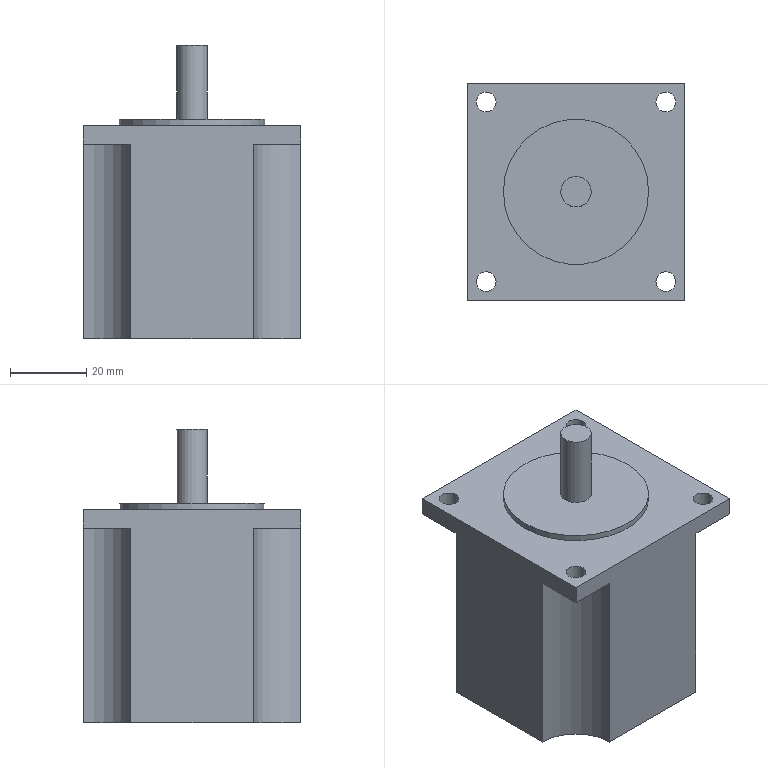Part | NX | features 57BYG350CL-SASSML-0601步进电机.SLDPRT 2 | 1 solid | 22 faces | box 57 x 57 x 76.9 mm | volume 158968 mm3 | plane 12 | cylinder 10 | commonest cylinder face diameters 5.2 x4 25 x4 8 x1 38.1 x1
STEP:
#1=CARTESIAN_POINT('',(-36.836,-5.583,23.));
#2=VERTEX_POINT('',#1);
#3=CARTESIAN_POINT('',(-36.836,26.417,23.));
#4=VERTEX_POINT('',#3);
#5=CARTESIAN_POINT('',(-36.836,38.917,23.));
#6=DIRECTION('',(0.,1.,0.));
#7=VECTOR('',#6,1000.);
#8=LINE('',#5,#7);
#9=EDGE_CURVE('',#2,#4,#8,.T.);
#10=ORIENTED_EDGE('',*,*,#9,.F.);
#11=CARTESIAN_POINT('',(-36.836,-5.583,74.));
#12=VERTEX_POINT('',#11);
#13=CARTESIAN_POINT('',(-36.836,-5.583,74.));
#14=DIRECTION('',(0.,0.,-1.));
#15=VECTOR('',#14,1000.);
#16=LINE('',#13,#15);
#17=EDGE_CURVE('',#2,#12,#16,.F.);
#18=ORIENTED_EDGE('',*,*,#17,.T.);
#19=CARTESIAN_POINT('',(-36.836,-18.083,74.));
#20=VERTEX_POINT('',#19);
#21=CARTESIAN_POINT('',(-36.836,-18.083,74.));
#22=DIRECTION('',(0.,1.,0.));
#23=VECTOR('',#22,1000.);
#24=LINE('',#21,#23);
#25=EDGE_CURVE('',#20,#12,#24,.T.);
#26=ORIENTED_EDGE('',*,*,#25,.F.);
#27=CARTESIAN_POINT('',(-36.836,-18.083,78.9));
#28=VERTEX_POINT('',#27);
#29=CARTESIAN_POINT('',(-36.836,-18.083,78.9));
#30=DIRECTION('',(0.,0.,-1.));
#31=VECTOR('',#30,1000.);
#32=LINE('',#29,#31);
#33=EDGE_CURVE('',#28,#20,#32,.T.);
#34=ORIENTED_EDGE('',*,*,#33,.F.);
#35=CARTESIAN_POINT('',(-36.836,38.917,78.9));
#36=VERTEX_POINT('',#35);
#37=CARTESIAN_POINT('',(-36.836,-18.083,78.9));
#38=DIRECTION('',(0.,-1.,0.));
#39=VECTOR('',#38,1000.);
#40=LINE('',#37,#39);
#41=EDGE_CURVE('',#36,#28,#40,.T.);
#42=ORIENTED_EDGE('',*,*,#41,.F.);
#43=CARTESIAN_POINT('',(-36.836,38.917,74.));
#44=VERTEX_POINT('',#43);
#45=CARTESIAN_POINT('',(-36.836,38.917,78.9));
#46=DIRECTION('',(0.,0.,-1.));
#47=VECTOR('',#46,1000.);
#48=LINE('',#45,#47);
#49=EDGE_CURVE('',#36,#44,#48,.T.);
#50=ORIENTED_EDGE('',*,*,#49,.T.);
#51=CARTESIAN_POINT('',(-36.836,26.417,74.));
#52=VERTEX_POINT('',#51);
#53=CARTESIAN_POINT('',(-36.836,-18.083,74.));
#54=DIRECTION('',(0.,1.,0.));
#55=VECTOR('',#54,1000.);
#56=LINE('',#53,#55);
#57=EDGE_CURVE('',#52,#44,#56,.T.);
#58=ORIENTED_EDGE('',*,*,#57,.F.);
#59=CARTESIAN_POINT('',(-36.836,26.417,74.));
#60=DIRECTION('',(0.,0.,-1.));
#61=VECTOR('',#60,1000.);
#62=LINE('',#59,#61);
#63=EDGE_CURVE('',#52,#4,#62,.T.);
#64=ORIENTED_EDGE('',*,*,#63,.T.);
#65=EDGE_LOOP('',(#10,#18,#26,#34,#42,#50,#58,#64));
#66=FACE_BOUND('',#65,.T.);
#67=CARTESIAN_POINT('',(-36.836,-18.083,78.9));
#68=DIRECTION('',(1.,0.,0.));
#69=DIRECTION('',(0.,0.,-1.));
#70=AXIS2_PLACEMENT_3D('',#67,#68,#69);
#71=PLANE('',#70);
#72=ADVANCED_FACE('',(#66),#71,.F.);
#73=CARTESIAN_POINT('',(7.664,-18.083,23.));
#74=VERTEX_POINT('',#73);
#75=CARTESIAN_POINT('',(-24.336,-18.083,23.));
#76=VERTEX_POINT('',#75);
#77=CARTESIAN_POINT('',(20.164,-18.083,23.));
#78=DIRECTION('',(-1.,0.,0.));
#79=VECTOR('',#78,1000.);
#80=LINE('',#77,#79);
#81=EDGE_CURVE('',#74,#76,#80,.T.);
#82=ORIENTED_EDGE('',*,*,#81,.F.);
#83=CARTESIAN_POINT('',(7.664,-18.083,74.));
#84=VERTEX_POINT('',#83);
#85=CARTESIAN_POINT('',(7.664,-18.083,74.));
#86=DIRECTION('',(0.,0.,-1.));
#87=VECTOR('',#86,1000.);
#88=LINE('',#85,#87);
#89=EDGE_CURVE('',#74,#84,#88,.F.);
#90=ORIENTED_EDGE('',*,*,#89,.T.);
#91=CARTESIAN_POINT('',(20.164,-18.083,74.));
#92=VERTEX_POINT('',#91);
#93=CARTESIAN_POINT('',(-36.836,-18.083,74.));
#94=DIRECTION('',(-1.,0.,0.));
#95=VECTOR('',#94,1000.);
#96=LINE('',#93,#95);
#97=EDGE_CURVE('',#92,#84,#96,.T.);
#98=ORIENTED_EDGE('',*,*,#97,.F.);
#99=CARTESIAN_POINT('',(20.164,-18.083,78.9));
#100=VERTEX_POINT('',#99);
#101=CARTESIAN_POINT('',(20.164,-18.083,78.9));
#102=DIRECTION('',(0.,0.,-1.));
#103=VECTOR('',#102,1000.);
#104=LINE('',#101,#103);
#105=EDGE_CURVE('',#100,#92,#104,.T.);
#106=ORIENTED_EDGE('',*,*,#105,.F.);
#107=CARTESIAN_POINT('',(-36.836,-18.083,78.9));
#108=DIRECTION('',(1.,0.,0.));
#109=VECTOR('',#108,1000.);
#110=LINE('',#107,#109);
#111=EDGE_CURVE('',#28,#100,#110,.T.);
#112=ORIENTED_EDGE('',*,*,#111,.F.);
#113=ORIENTED_EDGE('',*,*,#33,.T.);
#114=CARTESIAN_POINT('',(-24.336,-18.083,74.));
#115=VERTEX_POINT('',#114);
#116=CARTESIAN_POINT('',(-36.836,-18.083,74.));
#117=DIRECTION('',(-1.,0.,0.));
#118=VECTOR('',#117,1000.);
#119=LINE('',#116,#118);
#120=EDGE_CURVE('',#115,#20,#119,.T.);
#121=ORIENTED_EDGE('',*,*,#120,.F.);
#122=CARTESIAN_POINT('',(-24.336,-18.083,74.));
#123=DIRECTION('',(0.,0.,-1.));
#124=VECTOR('',#123,1000.);
#125=LINE('',#122,#124);
#126=EDGE_CURVE('',#115,#76,#125,.T.);
#127=ORIENTED_EDGE('',*,*,#126,.T.);
#128=EDGE_LOOP('',(#82,#90,#98,#106,#112,#113,#121,#127));
#129=FACE_BOUND('',#128,.T.);
#130=CARTESIAN_POINT('',(-36.836,-18.083,78.9));
#131=DIRECTION('',(0.,1.,0.));
#132=DIRECTION('',(0.,0.,1.));
#133=AXIS2_PLACEMENT_3D('',#130,#131,#132);
#134=PLANE('',#133);
#135=ADVANCED_FACE('',(#129),#134,.F.);
#136=CARTESIAN_POINT('',(20.164,26.417,23.));
#137=VERTEX_POINT('',#136);
#138=CARTESIAN_POINT('',(20.164,-5.583,23.));
#139=VERTEX_POINT('',#138);
#140=CARTESIAN_POINT('',(20.164,38.917,23.));
#141=DIRECTION('',(0.,-1.,0.));
#142=VECTOR('',#141,1000.);
#143=LINE('',#140,#142);
#144=EDGE_CURVE('',#137,#139,#143,.T.);
#145=ORIENTED_EDGE('',*,*,#144,.F.);
#146=CARTESIAN_POINT('',(20.164,26.417,74.));
#147=VERTEX_POINT('',#146);
#148=CARTESIAN_POINT('',(20.164,26.417,74.));
#149=DIRECTION('',(0.,0.,-1.));
#150=VECTOR('',#149,1000.);
#151=LINE('',#148,#150);
#152=EDGE_CURVE('',#137,#147,#151,.F.);
#153=ORIENTED_EDGE('',*,*,#152,.T.);
#154=CARTESIAN_POINT('',(20.164,38.917,74.));
#155=VERTEX_POINT('',#154);
#156=CARTESIAN_POINT('',(20.164,-18.083,74.));
#157=DIRECTION('',(0.,-1.,0.));
#158=VECTOR('',#157,1000.);
#159=LINE('',#156,#158);
#160=EDGE_CURVE('',#155,#147,#159,.T.);
#161=ORIENTED_EDGE('',*,*,#160,.F.);
#162=CARTESIAN_POINT('',(20.164,38.917,78.9));
#163=VERTEX_POINT('',#162);
#164=CARTESIAN_POINT('',(20.164,38.917,78.9));
#165=DIRECTION('',(0.,0.,-1.));
#166=VECTOR('',#165,1000.);
#167=LINE('',#164,#166);
#168=EDGE_CURVE('',#163,#155,#167,.T.);
#169=ORIENTED_EDGE('',*,*,#168,.F.);
#170=CARTESIAN_POINT('',(20.164,-18.083,78.9));
#171=DIRECTION('',(0.,1.,0.));
#172=VECTOR('',#171,1000.);
#173=LINE('',#170,#172);
#174=EDGE_CURVE('',#100,#163,#173,.T.);
#175=ORIENTED_EDGE('',*,*,#174,.F.);
#176=ORIENTED_EDGE('',*,*,#105,.T.);
#177=CARTESIAN_POINT('',(20.164,-5.583,74.));
#178=VERTEX_POINT('',#177);
#179=CARTESIAN_POINT('',(20.164,-18.083,74.));
#180=DIRECTION('',(0.,-1.,0.));
#181=VECTOR('',#180,1000.);
#182=LINE('',#179,#181);
#183=EDGE_CURVE('',#178,#92,#182,.T.);
#184=ORIENTED_EDGE('',*,*,#183,.F.);
#185=CARTESIAN_POINT('',(20.164,-5.583,74.));
#186=DIRECTION('',(0.,0.,-1.));
#187=VECTOR('',#186,1000.);
#188=LINE('',#185,#187);
#189=EDGE_CURVE('',#178,#139,#188,.T.);
#190=ORIENTED_EDGE('',*,*,#189,.T.);
#191=EDGE_LOOP('',(#145,#153,#161,#169,#175,#176,#184,#190));
#192=FACE_BOUND('',#191,.T.);
#193=CARTESIAN_POINT('',(20.164,-18.083,78.9));
#194=DIRECTION('',(-1.,0.,0.));
#195=DIRECTION('',(0.,0.,1.));
#196=AXIS2_PLACEMENT_3D('',#193,#194,#195);
#197=PLANE('',#196);
#198=ADVANCED_FACE('',(#192),#197,.F.);
#199=CARTESIAN_POINT('',(-24.336,38.917,23.));
#200=VERTEX_POINT('',#199);
#201=CARTESIAN_POINT('',(7.664,38.917,23.));
#202=VERTEX_POINT('',#201);
#203=CARTESIAN_POINT('',(20.164,38.917,23.));
#204=DIRECTION('',(1.,0.,0.));
#205=VECTOR('',#204,1000.);
#206=LINE('',#203,#205);
#207=EDGE_CURVE('',#200,#202,#206,.T.);
#208=ORIENTED_EDGE('',*,*,#207,.F.);
#209=CARTESIAN_POINT('',(-24.336,38.917,74.));
#210=VERTEX_POINT('',#209);
#211=CARTESIAN_POINT('',(-24.336,38.917,74.));
#212=DIRECTION('',(0.,0.,-1.));
#213=VECTOR('',#212,1000.);
#214=LINE('',#211,#213);
#215=EDGE_CURVE('',#200,#210,#214,.F.);
#216=ORIENTED_EDGE('',*,*,#215,.T.);
#217=CARTESIAN_POINT('',(-36.836,38.917,74.));
#218=DIRECTION('',(1.,0.,0.));
#219=VECTOR('',#218,1000.);
#220=LINE('',#217,#219);
#221=EDGE_CURVE('',#44,#210,#220,.T.);
#222=ORIENTED_EDGE('',*,*,#221,.F.);
#223=ORIENTED_EDGE('',*,*,#49,.F.);
#224=CARTESIAN_POINT('',(-36.836,38.917,78.9));
#225=DIRECTION('',(-1.,0.,0.));
#226=VECTOR('',#225,1000.);
#227=LINE('',#224,#226);
#228=EDGE_CURVE('',#163,#36,#227,.T.);
#229=ORIENTED_EDGE('',*,*,#228,.F.);
#230=ORIENTED_EDGE('',*,*,#168,.T.);
#231=CARTESIAN_POINT('',(7.664,38.917,74.));
#232=VERTEX_POINT('',#231);
#233=CARTESIAN_POINT('',(-36.836,38.917,74.));
#234=DIRECTION('',(1.,0.,0.));
#235=VECTOR('',#234,1000.);
#236=LINE('',#233,#235);
#237=EDGE_CURVE('',#232,#155,#236,.T.);
#238=ORIENTED_EDGE('',*,*,#237,.F.);
#239=CARTESIAN_POINT('',(7.664,38.917,74.));
#240=DIRECTION('',(0.,0.,-1.));
#241=VECTOR('',#240,1000.);
#242=LINE('',#239,#241);
#243=EDGE_CURVE('',#232,#202,#242,.T.);
#244=ORIENTED_EDGE('',*,*,#243,.T.);
#245=EDGE_LOOP('',(#208,#216,#222,#223,#229,#230,#238,#244));
#246=FACE_BOUND('',#245,.T.);
#247=CARTESIAN_POINT('',(-36.836,38.917,78.9));
#248=DIRECTION('',(0.,-1.,0.));
#249=DIRECTION('',(0.,0.,-1.));
#250=AXIS2_PLACEMENT_3D('',#247,#248,#249);
#251=PLANE('',#250);
#252=ADVANCED_FACE('',(#246),#251,.F.);
#253=CARTESIAN_POINT('',(20.164,38.917,23.));
#254=DIRECTION('',(0.,0.,-1.));
#255=DIRECTION('',(-1.,0.,0.));
#256=AXIS2_PLACEMENT_3D('',#253,#254,#255);
#257=CIRCLE('',#256,12.5);
#258=EDGE_CURVE('',#202,#137,#257,.F.);
#259=ORIENTED_EDGE('',*,*,#258,.F.);
#260=ORIENTED_EDGE('',*,*,#243,.F.);
#261=CARTESIAN_POINT('',(20.164,38.917,74.));
#262=DIRECTION('',(0.,0.,-1.));
#263=DIRECTION('',(-1.,0.,0.));
#264=AXIS2_PLACEMENT_3D('',#261,#262,#263);
#265=CIRCLE('',#264,12.5);
#266=EDGE_CURVE('',#147,#232,#265,.T.);
#267=ORIENTED_EDGE('',*,*,#266,.F.);
#268=ORIENTED_EDGE('',*,*,#152,.F.);
#269=EDGE_LOOP('',(#259,#260,#267,#268));
#270=FACE_BOUND('',#269,.T.);
#271=CARTESIAN_POINT('',(20.164,38.917,74.));
#272=DIRECTION('',(0.,0.,-1.));
#273=DIRECTION('',(-1.,0.,0.));
#274=AXIS2_PLACEMENT_3D('',#271,#272,#273);
#275=CYLINDRICAL_SURFACE('',#274,12.5);
#276=ADVANCED_FACE('',(#270),#275,.F.);
#277=CARTESIAN_POINT('',(20.164,-18.083,23.));
#278=DIRECTION('',(0.,0.,-1.));
#279=DIRECTION('',(-1.,0.,0.));
#280=AXIS2_PLACEMENT_3D('',#277,#278,#279);
#281=CIRCLE('',#280,12.5);
#282=EDGE_CURVE('',#139,#74,#281,.F.);
#283=ORIENTED_EDGE('',*,*,#282,.F.);
#284=ORIENTED_EDGE('',*,*,#189,.F.);
#285=CARTESIAN_POINT('',(20.164,-18.083,74.));
#286=DIRECTION('',(0.,0.,-1.));
#287=DIRECTION('',(-1.,0.,0.));
#288=AXIS2_PLACEMENT_3D('',#285,#286,#287);
#289=CIRCLE('',#288,12.5);
#290=EDGE_CURVE('',#84,#178,#289,.T.);
#291=ORIENTED_EDGE('',*,*,#290,.F.);
#292=ORIENTED_EDGE('',*,*,#89,.F.);
#293=EDGE_LOOP('',(#283,#284,#291,#292));
#294=FACE_BOUND('',#293,.T.);
#295=CARTESIAN_POINT('',(20.164,-18.083,74.));
#296=DIRECTION('',(0.,0.,-1.));
#297=DIRECTION('',(-1.,0.,0.));
#298=AXIS2_PLACEMENT_3D('',#295,#296,#297);
#299=CYLINDRICAL_SURFACE('',#298,12.5);
#300=ADVANCED_FACE('',(#294),#299,.F.);
#301=CARTESIAN_POINT('',(-36.836,-18.083,23.));
#302=DIRECTION('',(0.,0.,-1.));
#303=DIRECTION('',(-1.,0.,0.));
#304=AXIS2_PLACEMENT_3D('',#301,#302,#303);
#305=CIRCLE('',#304,12.5);
#306=EDGE_CURVE('',#76,#2,#305,.F.);
#307=ORIENTED_EDGE('',*,*,#306,.F.);
#308=ORIENTED_EDGE('',*,*,#126,.F.);
#309=CARTESIAN_POINT('',(-36.836,-18.083,74.));
#310=DIRECTION('',(0.,0.,-1.));
#311=DIRECTION('',(-1.,0.,0.));
#312=AXIS2_PLACEMENT_3D('',#309,#310,#311);
#313=CIRCLE('',#312,12.5);
#314=EDGE_CURVE('',#12,#115,#313,.T.);
#315=ORIENTED_EDGE('',*,*,#314,.F.);
#316=ORIENTED_EDGE('',*,*,#17,.F.);
#317=EDGE_LOOP('',(#307,#308,#315,#316));
#318=FACE_BOUND('',#317,.T.);
#319=CARTESIAN_POINT('',(-36.836,-18.083,74.));
#320=DIRECTION('',(0.,0.,-1.));
#321=DIRECTION('',(-1.,0.,0.));
#322=AXIS2_PLACEMENT_3D('',#319,#320,#321);
#323=CYLINDRICAL_SURFACE('',#322,12.5);
#324=ADVANCED_FACE('',(#318),#323,.F.);
#325=CARTESIAN_POINT('',(-36.836,38.917,23.));
#326=DIRECTION('',(0.,0.,-1.));
#327=DIRECTION('',(-1.,0.,0.));
#328=AXIS2_PLACEMENT_3D('',#325,#326,#327);
#329=CIRCLE('',#328,12.5);
#330=EDGE_CURVE('',#4,#200,#329,.F.);
#331=ORIENTED_EDGE('',*,*,#330,.F.);
#332=ORIENTED_EDGE('',*,*,#63,.F.);
#333=CARTESIAN_POINT('',(-36.836,38.917,74.));
#334=DIRECTION('',(0.,0.,-1.));
#335=DIRECTION('',(-1.,0.,0.));
#336=AXIS2_PLACEMENT_3D('',#333,#334,#335);
#337=CIRCLE('',#336,12.5);
#338=EDGE_CURVE('',#210,#52,#337,.T.);
#339=ORIENTED_EDGE('',*,*,#338,.F.);
#340=ORIENTED_EDGE('',*,*,#215,.F.);
#341=EDGE_LOOP('',(#331,#332,#339,#340));
#342=FACE_BOUND('',#341,.T.);
#343=CARTESIAN_POINT('',(-36.836,38.917,74.));
#344=DIRECTION('',(0.,0.,-1.));
#345=DIRECTION('',(-1.,0.,0.));
#346=AXIS2_PLACEMENT_3D('',#343,#344,#345);
#347=CYLINDRICAL_SURFACE('',#346,12.5);
#348=ADVANCED_FACE('',(#342),#347,.F.);
#349=CARTESIAN_POINT('',(-29.286,33.967,78.9));
#350=VERTEX_POINT('',#349);
#351=CARTESIAN_POINT('',(-31.886,33.967,78.9));
#352=DIRECTION('',(0.,0.,1.));
#353=DIRECTION('',(1.,0.,0.));
#354=AXIS2_PLACEMENT_3D('',#351,#352,#353);
#355=CIRCLE('',#354,2.6);
#356=EDGE_CURVE('',#350,#350,#355,.T.);
#357=ORIENTED_EDGE('',*,*,#356,.T.);
#358=EDGE_LOOP('',(#357));
#359=FACE_BOUND('',#358,.T.);
#360=CARTESIAN_POINT('',(-34.486,33.967,74.));
#361=VERTEX_POINT('',#360);
#362=CARTESIAN_POINT('',(-31.886,33.967,74.));
#363=DIRECTION('',(0.,0.,-1.));
#364=DIRECTION('',(-1.,0.,0.));
#365=AXIS2_PLACEMENT_3D('',#362,#363,#364);
#366=CIRCLE('',#365,2.6);
#367=EDGE_CURVE('',#361,#361,#366,.F.);
#368=ORIENTED_EDGE('',*,*,#367,.F.);
#369=EDGE_LOOP('',(#368));
#370=FACE_BOUND('',#369,.T.);
#371=CARTESIAN_POINT('',(-31.886,33.967,78.9));
#372=DIRECTION('',(0.,0.,1.));
#373=DIRECTION('',(1.,0.,0.));
#374=AXIS2_PLACEMENT_3D('',#371,#372,#373);
#375=CYLINDRICAL_SURFACE('',#374,2.6);
#376=ADVANCED_FACE('',(#359,#370),#375,.F.);
#377=CARTESIAN_POINT('',(-29.286,-13.133,78.9));
#378=VERTEX_POINT('',#377);
#379=CARTESIAN_POINT('',(-31.886,-13.133,78.9));
#380=DIRECTION('',(0.,0.,1.));
#381=DIRECTION('',(1.,0.,0.));
#382=AXIS2_PLACEMENT_3D('',#379,#380,#381);
#383=CIRCLE('',#382,2.6);
#384=EDGE_CURVE('',#378,#378,#383,.T.);
#385=ORIENTED_EDGE('',*,*,#384,.T.);
#386=EDGE_LOOP('',(#385));
#387=FACE_BOUND('',#386,.T.);
#388=CARTESIAN_POINT('',(-34.486,-13.133,74.));
#389=VERTEX_POINT('',#388);
#390=CARTESIAN_POINT('',(-31.886,-13.133,74.));
#391=DIRECTION('',(0.,0.,-1.));
#392=DIRECTION('',(-1.,0.,0.));
#393=AXIS2_PLACEMENT_3D('',#390,#391,#392);
#394=CIRCLE('',#393,2.6);
#395=EDGE_CURVE('',#389,#389,#394,.F.);
#396=ORIENTED_EDGE('',*,*,#395,.F.);
#397=EDGE_LOOP('',(#396));
#398=FACE_BOUND('',#397,.T.);
#399=CARTESIAN_POINT('',(-31.886,-13.133,78.9));
#400=DIRECTION('',(0.,0.,1.));
#401=DIRECTION('',(1.,0.,0.));
#402=AXIS2_PLACEMENT_3D('',#399,#400,#401);
#403=CYLINDRICAL_SURFACE('',#402,2.6);
#404=ADVANCED_FACE('',(#387,#398),#403,.F.);
#405=CARTESIAN_POINT('',(17.814,-13.133,78.9));
#406=VERTEX_POINT('',#405);
#407=CARTESIAN_POINT('',(15.214,-13.133,78.9));
#408=DIRECTION('',(0.,0.,1.));
#409=DIRECTION('',(1.,0.,0.));
#410=AXIS2_PLACEMENT_3D('',#407,#408,#409);
#411=CIRCLE('',#410,2.6);
#412=EDGE_CURVE('',#406,#406,#411,.T.);
#413=ORIENTED_EDGE('',*,*,#412,.T.);
#414=EDGE_LOOP('',(#413));
#415=FACE_BOUND('',#414,.T.);
#416=CARTESIAN_POINT('',(12.614,-13.133,74.));
#417=VERTEX_POINT('',#416);
#418=CARTESIAN_POINT('',(15.214,-13.133,74.));
#419=DIRECTION('',(0.,0.,-1.));
#420=DIRECTION('',(-1.,0.,0.));
#421=AXIS2_PLACEMENT_3D('',#418,#419,#420);
#422=CIRCLE('',#421,2.6);
#423=EDGE_CURVE('',#417,#417,#422,.F.);
#424=ORIENTED_EDGE('',*,*,#423,.F.);
#425=EDGE_LOOP('',(#424));
#426=FACE_BOUND('',#425,.T.);
#427=CARTESIAN_POINT('',(15.214,-13.133,78.9));
#428=DIRECTION('',(0.,0.,1.));
#429=DIRECTION('',(1.,0.,0.));
#430=AXIS2_PLACEMENT_3D('',#427,#428,#429);
#431=CYLINDRICAL_SURFACE('',#430,2.6);
#432=ADVANCED_FACE('',(#415,#426),#431,.F.);
#433=CARTESIAN_POINT('',(17.814,33.967,78.9));
#434=VERTEX_POINT('',#433);
#435=CARTESIAN_POINT('',(15.214,33.967,78.9));
#436=DIRECTION('',(0.,0.,1.));
#437=DIRECTION('',(1.,0.,0.));
#438=AXIS2_PLACEMENT_3D('',#435,#436,#437);
#439=CIRCLE('',#438,2.6);
#440=EDGE_CURVE('',#434,#434,#439,.T.);
#441=ORIENTED_EDGE('',*,*,#440,.T.);
#442=EDGE_LOOP('',(#441));
#443=FACE_BOUND('',#442,.T.);
#444=CARTESIAN_POINT('',(12.614,33.967,74.));
#445=VERTEX_POINT('',#444);
#446=CARTESIAN_POINT('',(15.214,33.967,74.));
#447=DIRECTION('',(0.,0.,-1.));
#448=DIRECTION('',(-1.,0.,0.));
#449=AXIS2_PLACEMENT_3D('',#446,#447,#448);
#450=CIRCLE('',#449,2.6);
#451=EDGE_CURVE('',#445,#445,#450,.F.);
#452=ORIENTED_EDGE('',*,*,#451,.F.);
#453=EDGE_LOOP('',(#452));
#454=FACE_BOUND('',#453,.T.);
#455=CARTESIAN_POINT('',(15.214,33.967,78.9));
#456=DIRECTION('',(0.,0.,1.));
#457=DIRECTION('',(1.,0.,0.));
#458=AXIS2_PLACEMENT_3D('',#455,#456,#457);
#459=CYLINDRICAL_SURFACE('',#458,2.6);
#460=ADVANCED_FACE('',(#443,#454),#459,.F.);
#461=CARTESIAN_POINT('',(10.714,10.417,80.5));
#462=VERTEX_POINT('',#461);
#463=CARTESIAN_POINT('',(-8.336,10.417,80.5));
#464=DIRECTION('',(0.,0.,1.));
#465=DIRECTION('',(1.,0.,0.));
#466=AXIS2_PLACEMENT_3D('',#463,#464,#465);
#467=CIRCLE('',#466,19.05);
#468=EDGE_CURVE('',#462,#462,#467,.T.);
#469=ORIENTED_EDGE('',*,*,#468,.T.);
#470=EDGE_LOOP('',(#469));
#471=FACE_BOUND('',#470,.T.);
#472=CARTESIAN_POINT('',(-4.336,10.417,80.5));
#473=VERTEX_POINT('',#472);
#474=CARTESIAN_POINT('',(-8.336,10.417,80.5));
#475=DIRECTION('',(0.,0.,1.));
#476=DIRECTION('',(1.,0.,0.));
#477=AXIS2_PLACEMENT_3D('',#474,#475,#476);
#478=CIRCLE('',#477,4.);
#479=EDGE_CURVE('',#473,#473,#478,.T.);
#480=ORIENTED_EDGE('',*,*,#479,.F.);
#481=EDGE_LOOP('',(#480));
#482=FACE_BOUND('',#481,.T.);
#483=CARTESIAN_POINT('',(-8.336,10.417,80.5));
#484=DIRECTION('',(0.,0.,1.));
#485=DIRECTION('',(1.,0.,0.));
#486=AXIS2_PLACEMENT_3D('',#483,#484,#485);
#487=PLANE('',#486);
#488=ADVANCED_FACE('',(#471,#482),#487,.T.);
#489=ORIENTED_EDGE('',*,*,#384,.F.);
#490=EDGE_LOOP('',(#489));
#491=FACE_BOUND('',#490,.T.);
#492=ORIENTED_EDGE('',*,*,#356,.F.);
#493=EDGE_LOOP('',(#492));
#494=FACE_BOUND('',#493,.T.);
#495=ORIENTED_EDGE('',*,*,#440,.F.);
#496=EDGE_LOOP('',(#495));
#497=FACE_BOUND('',#496,.T.);
#498=ORIENTED_EDGE('',*,*,#412,.F.);
#499=EDGE_LOOP('',(#498));
#500=FACE_BOUND('',#499,.T.);
#501=ORIENTED_EDGE('',*,*,#41,.T.);
#502=ORIENTED_EDGE('',*,*,#111,.T.);
#503=ORIENTED_EDGE('',*,*,#174,.T.);
#504=ORIENTED_EDGE('',*,*,#228,.T.);
#505=EDGE_LOOP('',(#501,#502,#503,#504));
#506=FACE_BOUND('',#505,.T.);
#507=CARTESIAN_POINT('',(-27.386,10.417,78.9));
#508=VERTEX_POINT('',#507);
#509=CARTESIAN_POINT('',(-8.336,10.417,78.9));
#510=DIRECTION('',(0.,0.,-1.));
#511=DIRECTION('',(-1.,0.,0.));
#512=AXIS2_PLACEMENT_3D('',#509,#510,#511);
#513=CIRCLE('',#512,19.05);
#514=EDGE_CURVE('',#508,#508,#513,.F.);
#515=ORIENTED_EDGE('',*,*,#514,.F.);
#516=EDGE_LOOP('',(#515));
#517=FACE_BOUND('',#516,.T.);
#518=CARTESIAN_POINT('',(-36.836,38.917,78.9));
#519=DIRECTION('',(0.,0.,-1.));
#520=DIRECTION('',(-1.,0.,0.));
#521=AXIS2_PLACEMENT_3D('',#518,#519,#520);
#522=PLANE('',#521);
#523=ADVANCED_FACE('',(#491,#494,#497,#500,#506,#517),#522,.F.);
#524=ORIENTED_EDGE('',*,*,#468,.F.);
#525=EDGE_LOOP('',(#524));
#526=FACE_BOUND('',#525,.T.);
#527=ORIENTED_EDGE('',*,*,#514,.T.);
#528=EDGE_LOOP('',(#527));
#529=FACE_BOUND('',#528,.T.);
#530=CARTESIAN_POINT('',(-8.336,10.417,80.5));
#531=DIRECTION('',(0.,0.,-1.));
#532=DIRECTION('',(-1.,0.,0.));
#533=AXIS2_PLACEMENT_3D('',#530,#531,#532);
#534=CYLINDRICAL_SURFACE('',#533,19.05);
#535=ADVANCED_FACE('',(#526,#529),#534,.T.);
#536=CARTESIAN_POINT('',(-4.336,10.417,99.9));
#537=VERTEX_POINT('',#536);
#538=CARTESIAN_POINT('',(-8.336,10.417,99.9));
#539=DIRECTION('',(0.,0.,1.));
#540=DIRECTION('',(1.,0.,0.));
#541=AXIS2_PLACEMENT_3D('',#538,#539,#540);
#542=CIRCLE('',#541,4.);
#543=EDGE_CURVE('',#537,#537,#542,.T.);
#544=ORIENTED_EDGE('',*,*,#543,.F.);
#545=EDGE_LOOP('',(#544));
#546=FACE_BOUND('',#545,.T.);
#547=ORIENTED_EDGE('',*,*,#479,.T.);
#548=EDGE_LOOP('',(#547));
#549=FACE_BOUND('',#548,.T.);
#550=CARTESIAN_POINT('',(-8.336,10.417,99.9));
#551=DIRECTION('',(0.,0.,-1.));
#552=DIRECTION('',(-1.,0.,0.));
#553=AXIS2_PLACEMENT_3D('',#550,#551,#552);
#554=CYLINDRICAL_SURFACE('',#553,4.);
#555=ADVANCED_FACE('',(#546,#549),#554,.T.);
#556=ORIENTED_EDGE('',*,*,#543,.T.);
#557=EDGE_LOOP('',(#556));
#558=FACE_BOUND('',#557,.T.);
#559=CARTESIAN_POINT('',(-8.336,10.417,99.9));
#560=DIRECTION('',(0.,0.,1.));
#561=DIRECTION('',(1.,0.,0.));
#562=AXIS2_PLACEMENT_3D('',#559,#560,#561);
#563=PLANE('',#562);
#564=ADVANCED_FACE('',(#558),#563,.T.);
#565=ORIENTED_EDGE('',*,*,#451,.T.);
#566=EDGE_LOOP('',(#565));
#567=FACE_BOUND('',#566,.T.);
#568=ORIENTED_EDGE('',*,*,#160,.T.);
#569=ORIENTED_EDGE('',*,*,#266,.T.);
#570=ORIENTED_EDGE('',*,*,#237,.T.);
#571=EDGE_LOOP('',(#568,#569,#570));
#572=FACE_BOUND('',#571,.T.);
#573=CARTESIAN_POINT('',(20.164,38.917,74.));
#574=DIRECTION('',(0.,0.,-1.));
#575=DIRECTION('',(-1.,0.,0.));
#576=AXIS2_PLACEMENT_3D('',#573,#574,#575);
#577=PLANE('',#576);
#578=ADVANCED_FACE('',(#567,#572),#577,.T.);
#579=ORIENTED_EDGE('',*,*,#423,.T.);
#580=EDGE_LOOP('',(#579));
#581=FACE_BOUND('',#580,.T.);
#582=ORIENTED_EDGE('',*,*,#97,.T.);
#583=ORIENTED_EDGE('',*,*,#290,.T.);
#584=ORIENTED_EDGE('',*,*,#183,.T.);
#585=EDGE_LOOP('',(#582,#583,#584));
#586=FACE_BOUND('',#585,.T.);
#587=CARTESIAN_POINT('',(20.164,-18.083,74.));
#588=DIRECTION('',(0.,0.,-1.));
#589=DIRECTION('',(-1.,0.,0.));
#590=AXIS2_PLACEMENT_3D('',#587,#588,#589);
#591=PLANE('',#590);
#592=ADVANCED_FACE('',(#581,#586),#591,.T.);
#593=ORIENTED_EDGE('',*,*,#395,.T.);
#594=EDGE_LOOP('',(#593));
#595=FACE_BOUND('',#594,.T.);
#596=ORIENTED_EDGE('',*,*,#25,.T.);
#597=ORIENTED_EDGE('',*,*,#314,.T.);
#598=ORIENTED_EDGE('',*,*,#120,.T.);
#599=EDGE_LOOP('',(#596,#597,#598));
#600=FACE_BOUND('',#599,.T.);
#601=CARTESIAN_POINT('',(-36.836,-18.083,74.));
#602=DIRECTION('',(0.,0.,-1.));
#603=DIRECTION('',(-1.,0.,0.));
#604=AXIS2_PLACEMENT_3D('',#601,#602,#603);
#605=PLANE('',#604);
#606=ADVANCED_FACE('',(#595,#600),#605,.T.);
#607=ORIENTED_EDGE('',*,*,#367,.T.);
#608=EDGE_LOOP('',(#607));
#609=FACE_BOUND('',#608,.T.);
#610=ORIENTED_EDGE('',*,*,#57,.T.);
#611=ORIENTED_EDGE('',*,*,#221,.T.);
#612=ORIENTED_EDGE('',*,*,#338,.T.);
#613=EDGE_LOOP('',(#610,#611,#612));
#614=FACE_BOUND('',#613,.T.);
#615=CARTESIAN_POINT('',(-36.836,38.917,74.));
#616=DIRECTION('',(0.,0.,-1.));
#617=DIRECTION('',(-1.,0.,0.));
#618=AXIS2_PLACEMENT_3D('',#615,#616,#617);
#619=PLANE('',#618);
#620=ADVANCED_FACE('',(#609,#614),#619,.T.);
#621=ORIENTED_EDGE('',*,*,#258,.T.);
#622=ORIENTED_EDGE('',*,*,#144,.T.);
#623=ORIENTED_EDGE('',*,*,#282,.T.);
#624=ORIENTED_EDGE('',*,*,#81,.T.);
#625=ORIENTED_EDGE('',*,*,#306,.T.);
#626=ORIENTED_EDGE('',*,*,#9,.T.);
#627=ORIENTED_EDGE('',*,*,#330,.T.);
#628=ORIENTED_EDGE('',*,*,#207,.T.);
#629=EDGE_LOOP('',(#621,#622,#623,#624,#625,#626,#627,#628));
#630=FACE_BOUND('',#629,.T.);
#631=CARTESIAN_POINT('',(20.164,-18.083,23.));
#632=DIRECTION('',(0.,0.,-1.));
#633=DIRECTION('',(-1.,0.,0.));
#634=AXIS2_PLACEMENT_3D('',#631,#632,#633);
#635=PLANE('',#634);
#636=ADVANCED_FACE('',(#630),#635,.T.);
#637=CLOSED_SHELL('',(#72,#135,#198,#252,#276,#300,#324,#348,#376,#404,#432,#460,#488,#523,#535,#555,#564,#578,#592,#606,#620,#636));
#638=MANIFOLD_SOLID_BREP('',#637);
#639=(LENGTH_UNIT()NAMED_UNIT(*)SI_UNIT(.MILLI.,.METRE.));
#640=UNCERTAINTY_MEASURE_WITH_UNIT(LENGTH_MEASURE(0.00001),#639,'','');
#641=(NAMED_UNIT(*)PLANE_ANGLE_UNIT()SI_UNIT($,.RADIAN.));
#642=(NAMED_UNIT(*)SI_UNIT($,.STERADIAN.)SOLID_ANGLE_UNIT());
#643=(GEOMETRIC_REPRESENTATION_CONTEXT(3)GLOBAL_UNCERTAINTY_ASSIGNED_CONTEXT((#640))GLOBAL_UNIT_ASSIGNED_CONTEXT((#639,#641,#642))REPRESENTATION_CONTEXT('',''));
#644=ADVANCED_BREP_SHAPE_REPRESENTATION('',(#638),#643);